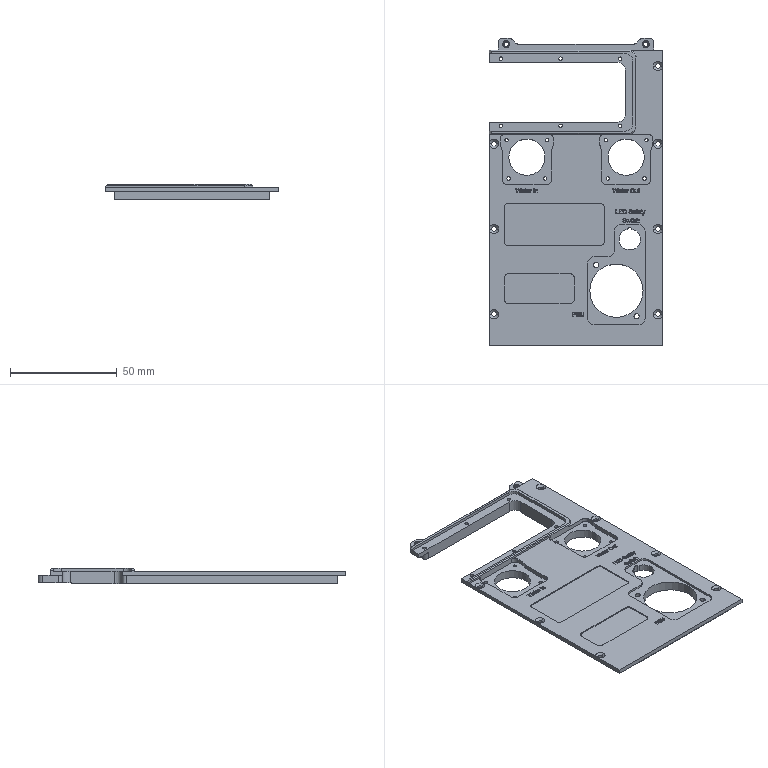CAM job | NX | 3-axis milling, drilling | part box 81.5 x 144.28 x 7.5 mm | stock box 85.22 x 147.78 x 10 mm
Tools:
number,name,description,diameter,corner_radius,flute_length,length,flutes
1,D6开粗,Milling Tool-5 Parameters,6.0,0.0,50.0,75.0,2
2,D4精光,Milling Tool-5 Parameters,4.0,0.0,50.0,75.0,2
3,倒角-3.,Drilling Tool,3.0,0.0,35.0,50.0,2
4,Z1.85,Drilling Tool,1.85,0.0,35.0,50.0,2
5,M2.,Drilling Tool,2.0,0.0,35.0,50.0,4
6,Z2.3,Drilling Tool,2.3,0.0,35.0,50.0,2
7,M2.5,Drilling Tool,2.5,0.0,35.0,50.0,4
8,Z2.5,Drilling Tool,2.5,0.0,35.0,50.0,2
9,M3,Drilling Tool,3.0,0.0,35.0,50.0,4
10,D2精光,Milling Tool-5 Parameters,2.0,0.0,50.0,75.0,2
13,SD-6.,Drilling Tool,6.0,0.0,35.0,50.0,2
0,D63面刀,Milling Tool-5 Parameters,63.0,0.0,50.0,75.0,2
0,D1D.5,Milling Tool-5 Parameters,1.5,0.0,50.0,75.0,2
0,D2.4钻头,Drilling Tool,2.4,0.0,35.0,50.0,2
Operations:
program,operation,operation_type,tool,method,geometry_group,spindle_rpm,surface_speed,feed_per_tooth,feed_cut,feed_plunge,cut_length_mm,path_length_mm,cut_time_min,machine_time_min
1,FLOOR_FACING,VolumeBased25DMillingOperation,D63面刀,METHOD,MCS_MAIN,4500.0,890.0,0.0889,800.0,100.0,481.109,575.109,0.6014,0.6108
1,DRILLING,Operation,倒角-3.,METHOD,WORKPIECE,3000.0,56.0,0.025,150.0,0.0,64.0,451.688,0.4267,0.4654
1,DRILLING_COPY_1,Operation,倒角-3.,METHOD,WORKPIECE,3000.0,56.0,0.025,150.0,0.0,8.6,106.769,0.0573,0.0672
1,DRILLING_COPY_1_COPY,Operation,Z2.3,METHOD,WORKPIECE,3000.0,21.0,0.0333,200.0,0.0,26.0,141.569,0.13,0.1416
1,DRILLING_COPY,Operation,Z1.85,METHOD,WORKPIECE,3000.0,17.0,0.0333,200.0,0.0,168.0,637.623,0.84,0.887
1,DRILLING_COPY_COPY,Operation,M2.,METHOD,WORKPIECE,300.0,1.0,0.1,0.4,0.0,147.0,595.623,367.5,367.545
1,DRILLING_COPY_1_COPY_COPY,Operation,M2.5,METHOD,WORKPIECE,300.0,2.0,0.1125,0.45,0.0,21.0,131.569,46.667,46.678
1,ADAPTIVE_MILLING,CavityMilling,D6开粗,METHOD,WORKPIECE,6500.0,122.0,0.1923,2500.0,100.0,20364.234,22391.265,8.041,8.243
1,PLANAR_MILL_COPY_1,PlanarMilling,D6开粗,METHOD,WORKPIECE,5000.0,94.0,0.07,700.0,100.0,377.932,479.732,0.5399,0.5501
1,PLANAR_MILL_COPY_2_COPY,PlanarMilling,D6开粗,METHOD,WORKPIECE,6000.0,113.0,0.2083,2500.0,100.0,609.155,717.155,0.2437,0.2545
1,CAVITY_MILL,CavityMilling,D6开粗,METHOD,WORKPIECE,6500.0,122.0,0.1923,2500.0,100.0,644.452,771.677,0.2578,0.2705
1,CAVITY_MILL_COPY_3,CavityMilling,D6开粗,METHOD,WORKPIECE,6500.0,122.0,0.1923,2500.0,100.0,294.685,394.084,0.1179,0.1278
1,FLOOR_WALL_COPY,VolumeBased25DMillingOperation,D6开粗,METHOD,WORKPIECE,6500.0,122.0,0.1923,2500.0,100.0,460.591,560.391,0.1842,0.1942
1,PLANAR_MILL_COPY_COPY_2_COPY_2_COPY,PlanarMilling,D4精光,METHOD,WORKPIECE,6000.0,113.0,0.0583,700.0,100.0,47.74,149.74,0.0682,0.0784
1,PLANAR_MILL_COPY_COPY_1_COPY_COPY_COPY_1_COPY_COPY_1_COPY_COPY_1_COPY_COPY,PlanarMilling,D4精光,METHOD,WORKPIECE,4500.0,56.0,0.0889,800.0,100.0,363.185,470.185,0.454,0.4647
1,CAVITY_MILL_COPY,CavityMilling,D4精光,METHOD,WORKPIECE,4500.0,56.0,0.0889,800.0,100.0,1282.093,2337.848,1.603,1.708
1,FLOOR_WALL,VolumeBased25DMillingOperation,D4精光,METHOD,WORKPIECE,4500.0,56.0,0.0889,800.0,100.0,2659.291,4195.609,3.324,3.478
1,FLOOR_WALL_COPY_1,VolumeBased25DMillingOperation,D4精光,METHOD,WORKPIECE,4500.0,56.0,0.0889,800.0,100.0,917.599,2507.408,1.147,1.306
1,PLANAR_MILL,PlanarMilling,D4精光,METHOD,WORKPIECE,4500.0,56.0,0.0889,800.0,100.0,195.409,743.505,0.2443,0.2991
1,PLANAR_MILL_COPY_1_COPY,PlanarMilling,D4精光,METHOD,WORKPIECE,4500.0,56.0,0.0889,800.0,100.0,752.806,948.285,0.941,0.9606
1,PLANAR_MILL_COPY_2_COPY_COPY,PlanarMilling,D4精光,METHOD,WORKPIECE,4500.0,56.0,0.0889,800.0,100.0,603.724,711.724,0.7547,0.7655
1,CAVITY_MILL_COPY_COPY,CavityMilling,D2精光,METHOD,WORKPIECE,6500.0,40.0,0.0923,1200.0,100.0,641.566,1454.373,0.5346,0.6159
1,CAVITY_MILL_COPY_1_COPY,CavityMilling,D2精光,METHOD,WORKPIECE,5500.0,122.0,0.1923,800.0,100.0,426.446,704.897,0.5331,0.5609
1,CAVITY_MILL_COPY_1_COPY_COPY_COPY,CavityMilling,D2精光,METHOD,WORKPIECE,5500.0,25.0,0.0273,300.0,100.0,426.446,704.897,1.421,1.449
1,PLANAR_MILL_COPY_COPY_1_COPY_COPY_COPY_1_COPY_COPY_1_COPY_COPY_1_COPY,PlanarMilling,D1D.5,METHOD,WORKPIECE,4500.0,21.0,0.0667,600.0,100.0,191.997,442.981,0.32,0.3451
1,CAVITY_MILL_COPY_1_COPY_COPY,CavityMilling,D1D.5,METHOD,WORKPIECE,5500.0,25.0,0.0273,300.0,100.0,29.525,138.525,0.0984,0.1093
1,PLANAR_MILL_COPY_COPY_1_COPY_COPY_COPY_COPY,PlanarMilling,倒角-3.,METHOD,WORKPIECE,6000.0,113.0,0.0583,700.0,100.0,393.707,491.707,0.5624,0.5722
1,PLANAR_MILL_COPY_COPY_1_COPY_COPY_COPY_1_COPY,PlanarMilling,倒角-3.,METHOD,WORKPIECE,6000.0,113.0,0.0583,700.0,100.0,668.443,970.473,0.9549,0.9851
1,PLANAR_MILL_COPY_COPY_1_COPY_COPY_COPY_1_COPY_COPY,PlanarMilling,倒角-3.,METHOD,WORKPIECE,6000.0,113.0,0.0583,700.0,100.0,117.054,211.454,0.1672,0.1767
1,PLANAR_MILL_COPY_COPY_1_COPY_COPY_COPY_1_COPY_COPY_COPY,PlanarMilling,倒角-3.,METHOD,WORKPIECE,6000.0,113.0,0.0583,700.0,100.0,135.469,229.869,0.1935,0.203
1,PLANAR_MILL_COPY_COPY_1_COPY_COPY_COPY_1_COPY_COPY_COPY_COPY,PlanarMilling,倒角-3.,METHOD,WORKPIECE,6000.0,113.0,0.0583,700.0,100.0,151.2,247.2,0.216,0.2256
1,PLANAR_MILL_COPY_COPY_1_COPY_COPY,PlanarMilling,倒角-3.,METHOD,WORKPIECE,6000.0,113.0,0.0583,700.0,100.0,346.352,450.352,0.4948,0.5052
1,PLANAR_MILL_COPY_COPY_1_COPY_COPY_COPY_1_COPY_COPY_1,PlanarMilling,倒角-3.,METHOD,WORKPIECE,6000.0,113.0,0.0583,700.0,100.0,165.149,261.149,0.2359,0.2455
1,PLANAR_MILL_COPY_COPY_1_COPY_COPY_COPY_1_COPY_COPY_1_COPY,PlanarMilling,倒角-3.,METHOD,WORKPIECE,6000.0,113.0,0.0583,700.0,100.0,80.122,179.122,0.1145,0.1244
1,PLANAR_MILL_COPY_COPY_1_COPY_COPY_COPY_1_COPY_COPY_1_COPY_COPY,PlanarMilling,倒角-3.,METHOD,WORKPIECE,6000.0,113.0,0.0583,700.0,100.0,20.921,119.921,0.0299,0.0398
1,PLANAR_MILL_COPY_COPY_1_COPY_COPY_COPY_1_COPY_COPY_1_COPY_COPY_1,PlanarMilling,倒角-3.,METHOD,WORKPIECE,6000.0,113.0,0.0583,700.0,100.0,33.77,135.77,0.0482,0.0584
1,DRILLING_COPY_2,Operation,倒角-3.,METHOD,WORKPIECE,3000.0,56.0,0.025,150.0,0.0,29.05,412.229,0.1937,0.232
1,DRILLING_COPY_2_COPY,Operation,倒角-3.,METHOD,WORKPIECE,3000.0,56.0,0.025,150.0,0.0,8.7,72.157,0.058,0.0643
1,DRILLING_COPY_2_COPY_COPY,Operation,Z2.5,METHOD,WORKPIECE,3000.0,23.0,0.0333,200.0,0.0,22.0,98.757,0.11,0.1177
1,DRILLING_COPY_2_COPY_COPY_1,Operation,M3,METHOD,WORKPIECE,300.0,2.0,0.125,0.5,0.0,19.0,92.757,38.0,38.007
1,PLANAR_MILL_COPY_1_COPY_COPY,PlanarMilling,D4精光,METHOD,WORKPIECE,4500.0,56.0,0.0889,800.0,100.0,683.009,879.274,0.8538,0.8734
G55,FLOOR_FACING_COPY,VolumeBased25DMillingOperation,D63面刀,METHOD,MCS,4500.0,890.0,0.0889,800.0,100.0,1924.438,2412.586,2.405,2.454
G55,CAVITY_MILL_COPY_2,CavityMilling,D6开粗,METHOD,WORKPIECE_1,6500.0,122.0,0.1923,2500.0,100.0,12105.397,13848.08,4.842,5.016
G55,FLOOR_WALL_1_COPY_1,VolumeBased25DMillingOperation,D6开粗,METHOD,WORKPIECE_1,5500.0,100.0,0.1178,800.0,100.0,2198.252,2295.152,2.748,2.757
G55,FLOOR_WALL_1,VolumeBased25DMillingOperation,D6开粗,METHOD,WORKPIECE_1,5500.0,100.0,0.1178,800.0,100.0,2198.252,2295.252,2.748,2.757
G55,PLANAR_MILL_1,PlanarMilling,D6开粗,METHOD,WORKPIECE_1,5000.0,94.0,0.07,700.0,100.0,99.5,200.5,0.1421,0.1522
G55,PLANAR_MILL_1_COPY_1,PlanarMilling,D6开粗,METHOD,WORKPIECE_1,5000.0,94.0,0.07,700.0,100.0,176.856,273.856,0.2527,0.2624
G55,PLANAR_MILL_1_COPY,PlanarMilling,D6开粗,METHOD,WORKPIECE_1,5000.0,94.0,0.07,700.0,100.0,62.894,162.774,0.0898,0.0998
G55,PLANAR_MILL_1_COPY_COPY,PlanarMilling,D6开粗,METHOD,WORKPIECE_1,5000.0,94.0,0.07,700.0,100.0,80.724,177.724,0.1153,0.125
G55,CAVITY_MILL_COPY_COPY_1,CavityMilling,D4精光,METHOD,WORKPIECE_1,6500.0,81.0,0.1538,2000.0,100.0,142.14,623.738,0.0711,0.1192
G55,FLOOR_WALL_1_COPY,VolumeBased25DMillingOperation,D4精光,METHOD,WORKPIECE_1,5000.0,62.0,0.07,700.0,100.0,1810.107,2627.113,2.586,2.668
G55,HOLE_MILLING,CylinderMilling,D2精光,METHOD,WORKPIECE_1,4500.0,28.0,0.0333,300.0,100.0,59.792,340.492,0.1993,0.2274
G55,DRILLING_1,Operation,SD-6.,METHOD,WORKPIECE_1,2000.0,37.0,0.0375,150.0,0.0,35.0,465.111,0.2333,0.2763
G55,DRILLING_1_COPY,Operation,SD-6.,METHOD,WORKPIECE_1,2000.0,37.0,0.0375,150.0,0.0,9.6,194.769,0.064,0.0825
G55,DRILLING_1_COPY_COPY,Operation,SD-6.,METHOD,WORKPIECE_1,2000.0,37.0,0.0375,150.0,0.0,9.2,157.157,0.0613,0.0761
G55,PLANAR_MILL_2_COPY_1,PlanarMilling,SD-6.,METHOD,WORKPIECE_1,6500.0,61.0,0.1154,800.0,100.0,78.0,149.501,0.0975,0.1047
G55,DRILLING_1_COPY_1,Operation,倒角-3.,METHOD,WORKPIECE_1,2000.0,37.0,0.0375,150.0,0.0,56.0,418.744,0.3733,0.4096
G55,PLANAR_MILL_2,PlanarMilling,倒角-3.,METHOD,WORKPIECE_1,6500.0,61.0,0.1154,1500.0,100.0,165.423,266.423,0.1103,0.1204
G55,PLANAR_MILL_2_COPY,PlanarMilling,倒角-3.,METHOD,WORKPIECE_1,6500.0,61.0,0.1154,1500.0,100.0,536.249,1211.536,0.3575,0.425
G55,PLANAR_MILL_2_COPY_COPY,PlanarMilling,倒角-3.,METHOD,WORKPIECE_1,6500.0,61.0,0.1154,1500.0,100.0,112.248,364.848,0.0748,0.1001
G55,PLANAR_MILL_2_COPY_COPY_COPY_1,PlanarMilling,倒角-3.,METHOD,WORKPIECE_1,6500.0,61.0,0.1154,1500.0,100.0,116.333,340.503,0.0776,0.1
G55,PLANAR_MILL_2_COPY_COPY_COPY,PlanarMilling,倒角-3.,METHOD,WORKPIECE_1,6500.0,61.0,0.1154,1500.0,100.0,344.751,443.751,0.2298,0.2397
G55,PLANAR_MILL_2_COPY_COPY_COPY_COPY,PlanarMilling,倒角-3.,METHOD,WORKPIECE_1,6500.0,61.0,0.1154,1500.0,100.0,186.114,282.514,0.1241,0.1337
G55,PLANAR_MILL_2_COPY_COPY_COPY_COPY_COPY_1,PlanarMilling,倒角-3.,METHOD,WORKPIECE_1,6500.0,61.0,0.1154,1500.0,100.0,173.76,270.16,0.1158,0.1255
G55,PLANAR_MILL_2_COPY_COPY_COPY_COPY_COPY,PlanarMilling,倒角-3.,METHOD,WORKPIECE_1,6500.0,61.0,0.1154,1500.0,100.0,86.958,188.958,0.058,0.0682
G55,DRILLING_1_COPY_2,Operation,D2.4钻头,METHOD,WORKPIECE_1,2000.0,15.0,0.0375,150.0,0.0,63.0,521.111,0.42,0.4658